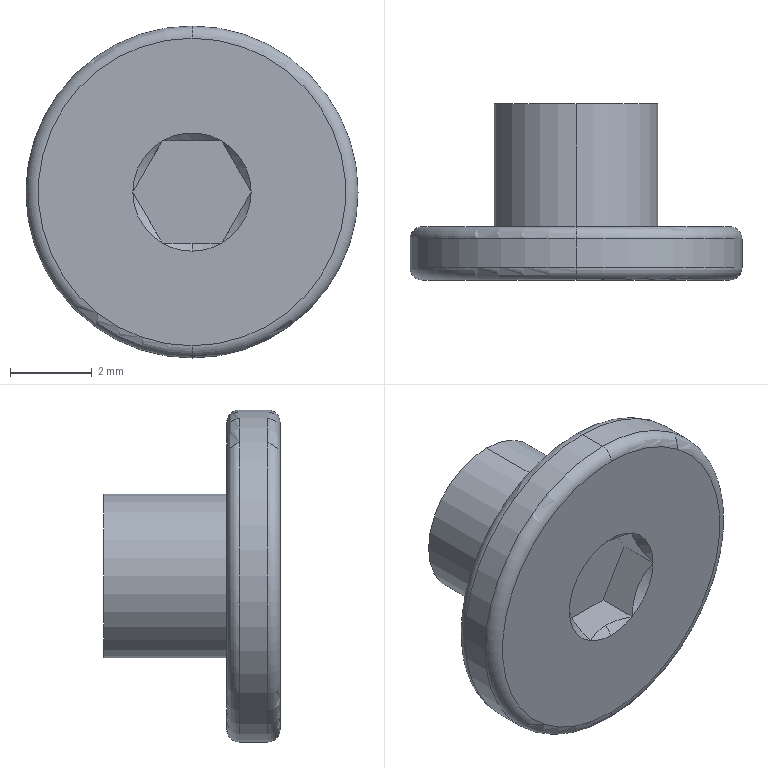Part | NX | features BREP 1 | 1 solid | 25 faces | box 8.1 x 4.3 x 8.1 mm | volume 98.194 mm3 | plane 10 | cone 7 | torus 4 | cylinder 4 | commonest cylinder face diameters 4 x2 8.1 x2
STEP:
#1=CARTESIAN_POINT('',(0.,0.1934,-1.25));
#2=VERTEX_POINT('',#1);
#3=CARTESIAN_POINT('',(0.7217,0.,-1.25));
#4=VERTEX_POINT('',#3);
#5=CARTESIAN_POINT('',(0.,0.1934,-1.25));
#6=CARTESIAN_POINT('',(0.2534,0.1934,-1.25));
#7=CARTESIAN_POINT('',(0.4959,0.1129,-1.25));
#8=CARTESIAN_POINT('',(0.7217,0.,-1.25));
#9=B_SPLINE_CURVE_WITH_KNOTS('',3,(#5,#6,#7,#8),.UNSPECIFIED.,.F.,.F.,(4,4),(0.,0.0007491),.UNSPECIFIED.);
#10=EDGE_CURVE('',#2,#4,#9,.T.);
#11=ORIENTED_EDGE('',*,*,#10,.F.);
#12=CARTESIAN_POINT('',(0.,0.,-1.443));
#13=VERTEX_POINT('',#12);
#14=CARTESIAN_POINT('',(0.,0.,-1.443));
#15=DIRECTION('',(0.,-0.7071,-0.7071));
#16=VECTOR('',#15,1000.);
#17=LINE('',#14,#16);
#18=EDGE_CURVE('',#2,#13,#17,.T.);
#19=ORIENTED_EDGE('',*,*,#18,.T.);
#20=CARTESIAN_POINT('',(0.,0.,0.));
#21=DIRECTION('',(0.,-1.,0.));
#22=DIRECTION('',(0.,0.,-1.));
#23=AXIS2_PLACEMENT_3D('',#20,#21,#22);
#24=CIRCLE('',#23,1.443);
#25=EDGE_CURVE('',#13,#4,#24,.T.);
#26=ORIENTED_EDGE('',*,*,#25,.T.);
#27=EDGE_LOOP('',(#11,#19,#26));
#28=FACE_BOUND('',#27,.T.);
#29=CARTESIAN_POINT('',(0.,0.,0.));
#30=DIRECTION('',(0.,-1.,0.));
#31=DIRECTION('',(0.,0.,1.));
#32=AXIS2_PLACEMENT_3D('',#29,#30,#31);
#33=CONICAL_SURFACE('',#32,1.443,0.7854);
#34=ADVANCED_FACE('',(#28),#33,.F.);
#35=CARTESIAN_POINT('',(0.,1.,-4.05));
#36=VERTEX_POINT('',#35);
#37=CARTESIAN_POINT('',(0.,1.,4.05));
#38=VERTEX_POINT('',#37);
#39=CARTESIAN_POINT('',(0.,1.,0.));
#40=DIRECTION('',(0.,-1.,0.));
#41=DIRECTION('',(0.,0.,1.));
#42=AXIS2_PLACEMENT_3D('',#39,#40,#41);
#43=CIRCLE('',#42,4.05);
#44=EDGE_CURVE('',#36,#38,#43,.T.);
#45=ORIENTED_EDGE('',*,*,#44,.F.);
#46=CARTESIAN_POINT('',(0.,1.3,-3.75));
#47=VERTEX_POINT('',#46);
#48=CARTESIAN_POINT('',(0.,1.,-3.75));
#49=DIRECTION('',(1.,0.,0.));
#50=DIRECTION('',(0.,0.,-1.));
#51=AXIS2_PLACEMENT_3D('',#48,#49,#50);
#52=CIRCLE('',#51,0.3);
#53=EDGE_CURVE('',#36,#47,#52,.T.);
#54=ORIENTED_EDGE('',*,*,#53,.T.);
#55=CARTESIAN_POINT('',(0.,1.3,3.75));
#56=VERTEX_POINT('',#55);
#57=CARTESIAN_POINT('',(0.,1.3,0.));
#58=DIRECTION('',(0.,1.,0.));
#59=DIRECTION('',(0.,0.,1.));
#60=AXIS2_PLACEMENT_3D('',#57,#58,#59);
#61=CIRCLE('',#60,3.75);
#62=EDGE_CURVE('',#56,#47,#61,.T.);
#63=ORIENTED_EDGE('',*,*,#62,.F.);
#64=CARTESIAN_POINT('',(0.,1.,3.75));
#65=DIRECTION('',(-1.,0.,0.));
#66=DIRECTION('',(0.,0.,1.));
#67=AXIS2_PLACEMENT_3D('',#64,#65,#66);
#68=CIRCLE('',#67,0.3);
#69=EDGE_CURVE('',#38,#56,#68,.T.);
#70=ORIENTED_EDGE('',*,*,#69,.F.);
#71=EDGE_LOOP('',(#45,#54,#63,#70));
#72=FACE_BOUND('',#71,.T.);
#73=CARTESIAN_POINT('',(0.,1.,0.));
#74=DIRECTION('',(0.,1.,0.));
#75=DIRECTION('',(0.,0.,-1.));
#76=AXIS2_PLACEMENT_3D('',#73,#74,#75);
#77=TOROIDAL_SURFACE('',#76,3.75,0.3);
#78=ADVANCED_FACE('',(#72),#77,.T.);
#79=CARTESIAN_POINT('',(0.,0.,-3.75));
#80=VERTEX_POINT('',#79);
#81=CARTESIAN_POINT('',(0.,0.,3.75));
#82=VERTEX_POINT('',#81);
#83=CARTESIAN_POINT('',(0.,0.,0.));
#84=DIRECTION('',(0.,-1.,0.));
#85=DIRECTION('',(0.,0.,1.));
#86=AXIS2_PLACEMENT_3D('',#83,#84,#85);
#87=CIRCLE('',#86,3.75);
#88=EDGE_CURVE('',#80,#82,#87,.T.);
#89=ORIENTED_EDGE('',*,*,#88,.F.);
#90=CARTESIAN_POINT('',(0.,0.3,-4.05));
#91=VERTEX_POINT('',#90);
#92=CARTESIAN_POINT('',(0.,0.3,-3.75));
#93=DIRECTION('',(1.,0.,0.));
#94=DIRECTION('',(0.,0.,-1.));
#95=AXIS2_PLACEMENT_3D('',#92,#93,#94);
#96=CIRCLE('',#95,0.3);
#97=EDGE_CURVE('',#80,#91,#96,.T.);
#98=ORIENTED_EDGE('',*,*,#97,.T.);
#99=CARTESIAN_POINT('',(0.,0.3,4.05));
#100=VERTEX_POINT('',#99);
#101=CARTESIAN_POINT('',(0.,0.3,0.));
#102=DIRECTION('',(0.,1.,0.));
#103=DIRECTION('',(0.,0.,1.));
#104=AXIS2_PLACEMENT_3D('',#101,#102,#103);
#105=CIRCLE('',#104,4.05);
#106=EDGE_CURVE('',#100,#91,#105,.T.);
#107=ORIENTED_EDGE('',*,*,#106,.F.);
#108=CARTESIAN_POINT('',(0.,0.3,3.75));
#109=DIRECTION('',(-1.,0.,0.));
#110=DIRECTION('',(0.,0.,1.));
#111=AXIS2_PLACEMENT_3D('',#108,#109,#110);
#112=CIRCLE('',#111,0.3);
#113=EDGE_CURVE('',#82,#100,#112,.T.);
#114=ORIENTED_EDGE('',*,*,#113,.F.);
#115=EDGE_LOOP('',(#89,#98,#107,#114));
#116=FACE_BOUND('',#115,.T.);
#117=CARTESIAN_POINT('',(0.,0.3,0.));
#118=DIRECTION('',(0.,1.,0.));
#119=DIRECTION('',(0.,0.,-1.));
#120=AXIS2_PLACEMENT_3D('',#117,#118,#119);
#121=TOROIDAL_SURFACE('',#120,3.75,0.3);
#122=ADVANCED_FACE('',(#116),#121,.T.);
#123=CARTESIAN_POINT('',(0.,4.3,2.));
#124=VERTEX_POINT('',#123);
#125=CARTESIAN_POINT('',(0.,4.3,-2.));
#126=VERTEX_POINT('',#125);
#127=CARTESIAN_POINT('',(0.,4.3,0.));
#128=DIRECTION('',(0.,1.,0.));
#129=DIRECTION('',(0.,0.,1.));
#130=AXIS2_PLACEMENT_3D('',#127,#128,#129);
#131=CIRCLE('',#130,2.);
#132=EDGE_CURVE('',#124,#126,#131,.T.);
#133=ORIENTED_EDGE('',*,*,#132,.F.);
#134=CARTESIAN_POINT('',(0.,1.3,2.));
#135=VERTEX_POINT('',#134);
#136=CARTESIAN_POINT('',(0.,4.3,2.));
#137=DIRECTION('',(0.,-1.,0.));
#138=VECTOR('',#137,1000.);
#139=LINE('',#136,#138);
#140=EDGE_CURVE('',#135,#124,#139,.F.);
#141=ORIENTED_EDGE('',*,*,#140,.F.);
#142=CARTESIAN_POINT('',(0.,1.3,-2.));
#143=VERTEX_POINT('',#142);
#144=CARTESIAN_POINT('',(0.,1.3,0.));
#145=DIRECTION('',(0.,1.,0.));
#146=DIRECTION('',(0.,0.,1.));
#147=AXIS2_PLACEMENT_3D('',#144,#145,#146);
#148=CIRCLE('',#147,2.);
#149=EDGE_CURVE('',#135,#143,#148,.T.);
#150=ORIENTED_EDGE('',*,*,#149,.T.);
#151=CARTESIAN_POINT('',(0.,4.3,-2.));
#152=DIRECTION('',(0.,-1.,0.));
#153=VECTOR('',#152,1000.);
#154=LINE('',#151,#153);
#155=EDGE_CURVE('',#143,#126,#154,.F.);
#156=ORIENTED_EDGE('',*,*,#155,.T.);
#157=EDGE_LOOP('',(#133,#141,#150,#156));
#158=FACE_BOUND('',#157,.T.);
#159=CARTESIAN_POINT('',(0.,4.3,0.));
#160=DIRECTION('',(0.,-1.,0.));
#161=DIRECTION('',(0.,0.,1.));
#162=AXIS2_PLACEMENT_3D('',#159,#160,#161);
#163=CYLINDRICAL_SURFACE('',#162,2.);
#164=ADVANCED_FACE('',(#158),#163,.T.);
#165=ORIENTED_EDGE('',*,*,#44,.T.);
#166=CARTESIAN_POINT('',(0.,1.3,4.05));
#167=DIRECTION('',(0.,-1.,0.));
#168=VECTOR('',#167,1000.);
#169=LINE('',#166,#168);
#170=EDGE_CURVE('',#100,#38,#169,.F.);
#171=ORIENTED_EDGE('',*,*,#170,.F.);
#172=ORIENTED_EDGE('',*,*,#106,.T.);
#173=CARTESIAN_POINT('',(0.,1.3,-4.05));
#174=DIRECTION('',(0.,-1.,0.));
#175=VECTOR('',#174,1000.);
#176=LINE('',#173,#175);
#177=EDGE_CURVE('',#91,#36,#176,.F.);
#178=ORIENTED_EDGE('',*,*,#177,.T.);
#179=EDGE_LOOP('',(#165,#171,#172,#178));
#180=FACE_BOUND('',#179,.T.);
#181=CARTESIAN_POINT('',(0.,1.3,0.));
#182=DIRECTION('',(0.,-1.,0.));
#183=DIRECTION('',(0.,0.,1.));
#184=AXIS2_PLACEMENT_3D('',#181,#182,#183);
#185=CYLINDRICAL_SURFACE('',#184,4.05);
#186=ADVANCED_FACE('',(#180),#185,.T.);
#187=ORIENTED_EDGE('',*,*,#170,.T.);
#188=CARTESIAN_POINT('',(0.,1.,0.));
#189=DIRECTION('',(0.,-1.,0.));
#190=DIRECTION('',(0.,0.,1.));
#191=AXIS2_PLACEMENT_3D('',#188,#189,#190);
#192=CIRCLE('',#191,4.05);
#193=EDGE_CURVE('',#38,#36,#192,.T.);
#194=ORIENTED_EDGE('',*,*,#193,.T.);
#195=ORIENTED_EDGE('',*,*,#177,.F.);
#196=CARTESIAN_POINT('',(0.,0.3,0.));
#197=DIRECTION('',(0.,1.,0.));
#198=DIRECTION('',(0.,0.,1.));
#199=AXIS2_PLACEMENT_3D('',#196,#197,#198);
#200=CIRCLE('',#199,4.05);
#201=EDGE_CURVE('',#91,#100,#200,.T.);
#202=ORIENTED_EDGE('',*,*,#201,.T.);
#203=EDGE_LOOP('',(#187,#194,#195,#202));
#204=FACE_BOUND('',#203,.T.);
#205=CARTESIAN_POINT('',(0.,1.3,0.));
#206=DIRECTION('',(0.,-1.,0.));
#207=DIRECTION('',(0.,0.,1.));
#208=AXIS2_PLACEMENT_3D('',#205,#206,#207);
#209=CYLINDRICAL_SURFACE('',#208,4.05);
#210=ADVANCED_FACE('',(#204),#209,.T.);
#211=ORIENTED_EDGE('',*,*,#62,.T.);
#212=CARTESIAN_POINT('',(0.,1.3,0.));
#213=DIRECTION('',(0.,1.,0.));
#214=DIRECTION('',(0.,0.,1.));
#215=AXIS2_PLACEMENT_3D('',#212,#213,#214);
#216=CIRCLE('',#215,3.75);
#217=EDGE_CURVE('',#47,#56,#216,.T.);
#218=ORIENTED_EDGE('',*,*,#217,.T.);
#219=EDGE_LOOP('',(#211,#218));
#220=FACE_BOUND('',#219,.T.);
#221=CARTESIAN_POINT('',(0.,1.3,0.));
#222=DIRECTION('',(0.,1.,0.));
#223=DIRECTION('',(0.,0.,1.));
#224=AXIS2_PLACEMENT_3D('',#221,#222,#223);
#225=CIRCLE('',#224,2.);
#226=EDGE_CURVE('',#143,#135,#225,.T.);
#227=ORIENTED_EDGE('',*,*,#226,.F.);
#228=ORIENTED_EDGE('',*,*,#149,.F.);
#229=EDGE_LOOP('',(#227,#228));
#230=FACE_BOUND('',#229,.T.);
#231=CARTESIAN_POINT('',(0.,1.3,0.));
#232=DIRECTION('',(0.,1.,0.));
#233=DIRECTION('',(-1.,0.,0.));
#234=AXIS2_PLACEMENT_3D('',#231,#232,#233);
#235=PLANE('',#234);
#236=ADVANCED_FACE('',(#220,#230),#235,.T.);
#237=CARTESIAN_POINT('',(0.,0.,0.));
#238=DIRECTION('',(0.,-1.,0.));
#239=DIRECTION('',(0.,0.,1.));
#240=AXIS2_PLACEMENT_3D('',#237,#238,#239);
#241=CIRCLE('',#240,3.75);
#242=EDGE_CURVE('',#82,#80,#241,.T.);
#243=ORIENTED_EDGE('',*,*,#242,.T.);
#244=ORIENTED_EDGE('',*,*,#88,.T.);
#245=EDGE_LOOP('',(#243,#244));
#246=FACE_BOUND('',#245,.T.);
#247=CARTESIAN_POINT('',(0.7217,0.,1.25));
#248=VERTEX_POINT('',#247);
#249=CARTESIAN_POINT('',(-0.7217,0.,1.25));
#250=VERTEX_POINT('',#249);
#251=CARTESIAN_POINT('',(0.,0.,0.));
#252=DIRECTION('',(0.,-1.,0.));
#253=DIRECTION('',(0.,0.,-1.));
#254=AXIS2_PLACEMENT_3D('',#251,#252,#253);
#255=CIRCLE('',#254,1.443);
#256=EDGE_CURVE('',#248,#250,#255,.T.);
#257=ORIENTED_EDGE('',*,*,#256,.F.);
#258=CARTESIAN_POINT('',(1.443,0.,0.));
#259=VERTEX_POINT('',#258);
#260=CARTESIAN_POINT('',(0.,0.,0.));
#261=DIRECTION('',(0.,-1.,0.));
#262=DIRECTION('',(0.,0.,-1.));
#263=AXIS2_PLACEMENT_3D('',#260,#261,#262);
#264=CIRCLE('',#263,1.443);
#265=EDGE_CURVE('',#259,#248,#264,.T.);
#266=ORIENTED_EDGE('',*,*,#265,.F.);
#267=CARTESIAN_POINT('',(0.,0.,0.));
#268=DIRECTION('',(0.,-1.,0.));
#269=DIRECTION('',(0.,0.,-1.));
#270=AXIS2_PLACEMENT_3D('',#267,#268,#269);
#271=CIRCLE('',#270,1.443);
#272=EDGE_CURVE('',#4,#259,#271,.T.);
#273=ORIENTED_EDGE('',*,*,#272,.F.);
#274=ORIENTED_EDGE('',*,*,#25,.F.);
#275=CARTESIAN_POINT('',(-0.7217,0.,-1.25));
#276=VERTEX_POINT('',#275);
#277=CARTESIAN_POINT('',(0.,0.,0.));
#278=DIRECTION('',(0.,-1.,0.));
#279=DIRECTION('',(0.,0.,-1.));
#280=AXIS2_PLACEMENT_3D('',#277,#278,#279);
#281=CIRCLE('',#280,1.443);
#282=EDGE_CURVE('',#276,#13,#281,.T.);
#283=ORIENTED_EDGE('',*,*,#282,.F.);
#284=CARTESIAN_POINT('',(-1.443,0.,0.));
#285=VERTEX_POINT('',#284);
#286=CARTESIAN_POINT('',(0.,0.,0.));
#287=DIRECTION('',(0.,-1.,0.));
#288=DIRECTION('',(0.,0.,-1.));
#289=AXIS2_PLACEMENT_3D('',#286,#287,#288);
#290=CIRCLE('',#289,1.443);
#291=EDGE_CURVE('',#285,#276,#290,.T.);
#292=ORIENTED_EDGE('',*,*,#291,.F.);
#293=CARTESIAN_POINT('',(0.,0.,0.));
#294=DIRECTION('',(0.,-1.,0.));
#295=DIRECTION('',(0.,0.,-1.));
#296=AXIS2_PLACEMENT_3D('',#293,#294,#295);
#297=CIRCLE('',#296,1.443);
#298=EDGE_CURVE('',#250,#285,#297,.T.);
#299=ORIENTED_EDGE('',*,*,#298,.F.);
#300=EDGE_LOOP('',(#257,#266,#273,#274,#283,#292,#299));
#301=FACE_BOUND('',#300,.T.);
#302=CARTESIAN_POINT('',(0.,0.,0.));
#303=DIRECTION('',(0.,1.,0.));
#304=DIRECTION('',(-1.,0.,0.));
#305=AXIS2_PLACEMENT_3D('',#302,#303,#304);
#306=PLANE('',#305);
#307=ADVANCED_FACE('',(#246,#301),#306,.F.);
#308=ORIENTED_EDGE('',*,*,#140,.T.);
#309=CARTESIAN_POINT('',(0.,4.3,0.));
#310=DIRECTION('',(0.,1.,0.));
#311=DIRECTION('',(0.,0.,1.));
#312=AXIS2_PLACEMENT_3D('',#309,#310,#311);
#313=CIRCLE('',#312,2.);
#314=EDGE_CURVE('',#126,#124,#313,.T.);
#315=ORIENTED_EDGE('',*,*,#314,.F.);
#316=ORIENTED_EDGE('',*,*,#155,.F.);
#317=ORIENTED_EDGE('',*,*,#226,.T.);
#318=EDGE_LOOP('',(#308,#315,#316,#317));
#319=FACE_BOUND('',#318,.T.);
#320=CARTESIAN_POINT('',(0.,4.3,0.));
#321=DIRECTION('',(0.,-1.,0.));
#322=DIRECTION('',(0.,0.,1.));
#323=AXIS2_PLACEMENT_3D('',#320,#321,#322);
#324=CYLINDRICAL_SURFACE('',#323,2.);
#325=ADVANCED_FACE('',(#319),#324,.T.);
#326=ORIENTED_EDGE('',*,*,#314,.T.);
#327=ORIENTED_EDGE('',*,*,#132,.T.);
#328=EDGE_LOOP('',(#326,#327));
#329=FACE_BOUND('',#328,.T.);
#330=CARTESIAN_POINT('',(0.,4.3,0.));
#331=DIRECTION('',(0.,1.,0.));
#332=DIRECTION('',(-1.,0.,0.));
#333=AXIS2_PLACEMENT_3D('',#330,#331,#332);
#334=PLANE('',#333);
#335=ADVANCED_FACE('',(#329),#334,.T.);
#336=ORIENTED_EDGE('',*,*,#97,.F.);
#337=ORIENTED_EDGE('',*,*,#242,.F.);
#338=ORIENTED_EDGE('',*,*,#113,.T.);
#339=ORIENTED_EDGE('',*,*,#201,.F.);
#340=EDGE_LOOP('',(#336,#337,#338,#339));
#341=FACE_BOUND('',#340,.T.);
#342=CARTESIAN_POINT('',(0.,0.3,0.));
#343=DIRECTION('',(0.,1.,0.));
#344=DIRECTION('',(0.,0.,-1.));
#345=AXIS2_PLACEMENT_3D('',#342,#343,#344);
#346=TOROIDAL_SURFACE('',#345,3.75,0.3);
#347=ADVANCED_FACE('',(#341),#346,.T.);
#348=ORIENTED_EDGE('',*,*,#53,.F.);
#349=ORIENTED_EDGE('',*,*,#193,.F.);
#350=ORIENTED_EDGE('',*,*,#69,.T.);
#351=ORIENTED_EDGE('',*,*,#217,.F.);
#352=EDGE_LOOP('',(#348,#349,#350,#351));
#353=FACE_BOUND('',#352,.T.);
#354=CARTESIAN_POINT('',(0.,1.,0.));
#355=DIRECTION('',(0.,1.,0.));
#356=DIRECTION('',(0.,0.,-1.));
#357=AXIS2_PLACEMENT_3D('',#354,#355,#356);
#358=TOROIDAL_SURFACE('',#357,3.75,0.3);
#359=ADVANCED_FACE('',(#353),#358,.T.);
#360=ORIENTED_EDGE('',*,*,#265,.T.);
#361=CARTESIAN_POINT('',(1.443,0.,0.));
#362=CARTESIAN_POINT('',(1.218,0.2255,0.3907));
#363=CARTESIAN_POINT('',(0.9486,0.2269,0.857));
#364=CARTESIAN_POINT('',(0.7217,0.,1.25));
#365=B_SPLINE_CURVE_WITH_KNOTS('',3,(#361,#362,#363,#364),.UNSPECIFIED.,.F.,.F.,(4,4),(0.,0.001491),.UNSPECIFIED.);
#366=EDGE_CURVE('',#259,#248,#365,.T.);
#367=ORIENTED_EDGE('',*,*,#366,.F.);
#368=EDGE_LOOP('',(#360,#367));
#369=FACE_BOUND('',#368,.T.);
#370=CARTESIAN_POINT('',(0.,0.,0.));
#371=DIRECTION('',(0.,-1.,0.));
#372=DIRECTION('',(0.,0.,1.));
#373=AXIS2_PLACEMENT_3D('',#370,#371,#372);
#374=CONICAL_SURFACE('',#373,1.443,0.7854);
#375=ADVANCED_FACE('',(#369),#374,.F.);
#376=ORIENTED_EDGE('',*,*,#256,.T.);
#377=CARTESIAN_POINT('',(0.7217,0.,1.25));
#378=CARTESIAN_POINT('',(0.2706,0.2255,1.25));
#379=CARTESIAN_POINT('',(-0.2679,0.2269,1.25));
#380=CARTESIAN_POINT('',(-0.7217,0.,1.25));
#381=B_SPLINE_CURVE_WITH_KNOTS('',3,(#377,#378,#379,#380),.UNSPECIFIED.,.F.,.F.,(4,4),(0.,0.001491),.UNSPECIFIED.);
#382=EDGE_CURVE('',#248,#250,#381,.T.);
#383=ORIENTED_EDGE('',*,*,#382,.F.);
#384=EDGE_LOOP('',(#376,#383));
#385=FACE_BOUND('',#384,.T.);
#386=CARTESIAN_POINT('',(0.,0.,0.));
#387=DIRECTION('',(0.,-1.,0.));
#388=DIRECTION('',(0.,0.,1.));
#389=AXIS2_PLACEMENT_3D('',#386,#387,#388);
#390=CONICAL_SURFACE('',#389,1.443,0.7854);
#391=ADVANCED_FACE('',(#385),#390,.F.);
#392=ORIENTED_EDGE('',*,*,#298,.T.);
#393=CARTESIAN_POINT('',(-0.7217,0.,1.25));
#394=CARTESIAN_POINT('',(-0.9472,0.2255,0.8593));
#395=CARTESIAN_POINT('',(-1.216,0.2269,0.393));
#396=CARTESIAN_POINT('',(-1.443,0.,0.));
#397=B_SPLINE_CURVE_WITH_KNOTS('',3,(#393,#394,#395,#396),.UNSPECIFIED.,.F.,.F.,(4,4),(0.,0.001491),.UNSPECIFIED.);
#398=EDGE_CURVE('',#250,#285,#397,.T.);
#399=ORIENTED_EDGE('',*,*,#398,.F.);
#400=EDGE_LOOP('',(#392,#399));
#401=FACE_BOUND('',#400,.T.);
#402=CARTESIAN_POINT('',(0.,0.,0.));
#403=DIRECTION('',(0.,-1.,0.));
#404=DIRECTION('',(0.,0.,1.));
#405=AXIS2_PLACEMENT_3D('',#402,#403,#404);
#406=CONICAL_SURFACE('',#405,1.443,0.7854);
#407=ADVANCED_FACE('',(#401),#406,.F.);
#408=ORIENTED_EDGE('',*,*,#291,.T.);
#409=CARTESIAN_POINT('',(-1.443,0.,0.));
#410=CARTESIAN_POINT('',(-1.218,0.2255,-0.3907));
#411=CARTESIAN_POINT('',(-0.9486,0.2269,-0.857));
#412=CARTESIAN_POINT('',(-0.7217,0.,-1.25));
#413=B_SPLINE_CURVE_WITH_KNOTS('',3,(#409,#410,#411,#412),.UNSPECIFIED.,.F.,.F.,(4,4),(0.,0.001491),.UNSPECIFIED.);
#414=EDGE_CURVE('',#285,#276,#413,.T.);
#415=ORIENTED_EDGE('',*,*,#414,.F.);
#416=EDGE_LOOP('',(#408,#415));
#417=FACE_BOUND('',#416,.T.);
#418=CARTESIAN_POINT('',(0.,0.,0.));
#419=DIRECTION('',(0.,-1.,0.));
#420=DIRECTION('',(0.,0.,1.));
#421=AXIS2_PLACEMENT_3D('',#418,#419,#420);
#422=CONICAL_SURFACE('',#421,1.443,0.7854);
#423=ADVANCED_FACE('',(#417),#422,.F.);
#424=ORIENTED_EDGE('',*,*,#18,.F.);
#425=CARTESIAN_POINT('',(-0.7217,0.,-1.25));
#426=CARTESIAN_POINT('',(-0.4955,0.1131,-1.25));
#427=CARTESIAN_POINT('',(-0.2554,0.1934,-1.25));
#428=CARTESIAN_POINT('',(0.,0.1934,-1.25));
#429=B_SPLINE_CURVE_WITH_KNOTS('',3,(#425,#426,#427,#428),.UNSPECIFIED.,.F.,.F.,(4,4),(0.,0.0007476),.UNSPECIFIED.);
#430=EDGE_CURVE('',#276,#2,#429,.T.);
#431=ORIENTED_EDGE('',*,*,#430,.F.);
#432=ORIENTED_EDGE('',*,*,#282,.T.);
#433=EDGE_LOOP('',(#424,#431,#432));
#434=FACE_BOUND('',#433,.T.);
#435=CARTESIAN_POINT('',(0.,0.,0.));
#436=DIRECTION('',(0.,-1.,0.));
#437=DIRECTION('',(0.,0.,1.));
#438=AXIS2_PLACEMENT_3D('',#435,#436,#437);
#439=CONICAL_SURFACE('',#438,1.443,0.7854);
#440=ADVANCED_FACE('',(#434),#439,.F.);
#441=ORIENTED_EDGE('',*,*,#272,.T.);
#442=CARTESIAN_POINT('',(0.7217,0.,-1.25));
#443=CARTESIAN_POINT('',(0.9472,0.2255,-0.8593));
#444=CARTESIAN_POINT('',(1.216,0.2269,-0.393));
#445=CARTESIAN_POINT('',(1.443,0.,0.));
#446=B_SPLINE_CURVE_WITH_KNOTS('',3,(#442,#443,#444,#445),.UNSPECIFIED.,.F.,.F.,(4,4),(0.,0.001491),.UNSPECIFIED.);
#447=EDGE_CURVE('',#4,#259,#446,.T.);
#448=ORIENTED_EDGE('',*,*,#447,.F.);
#449=EDGE_LOOP('',(#441,#448));
#450=FACE_BOUND('',#449,.T.);
#451=CARTESIAN_POINT('',(0.,0.,0.));
#452=DIRECTION('',(0.,-1.,0.));
#453=DIRECTION('',(0.,0.,1.));
#454=AXIS2_PLACEMENT_3D('',#451,#452,#453);
#455=CONICAL_SURFACE('',#454,1.443,0.7854);
#456=ADVANCED_FACE('',(#450),#455,.F.);
#457=CARTESIAN_POINT('',(0.7217,1.,-1.25));
#458=VERTEX_POINT('',#457);
#459=CARTESIAN_POINT('',(1.443,1.,0.));
#460=VERTEX_POINT('',#459);
#461=CARTESIAN_POINT('',(0.7217,1.,-1.25));
#462=DIRECTION('',(0.5,0.,0.866));
#463=VECTOR('',#462,1000.);
#464=LINE('',#461,#463);
#465=EDGE_CURVE('',#458,#460,#464,.T.);
#466=ORIENTED_EDGE('',*,*,#465,.T.);
#467=CARTESIAN_POINT('',(0.7217,1.,1.25));
#468=VERTEX_POINT('',#467);
#469=CARTESIAN_POINT('',(1.443,1.,0.));
#470=DIRECTION('',(-0.5,0.,0.866));
#471=VECTOR('',#470,1000.);
#472=LINE('',#469,#471);
#473=EDGE_CURVE('',#460,#468,#472,.T.);
#474=ORIENTED_EDGE('',*,*,#473,.T.);
#475=CARTESIAN_POINT('',(-0.7217,1.,1.25));
#476=VERTEX_POINT('',#475);
#477=CARTESIAN_POINT('',(0.7217,1.,1.25));
#478=DIRECTION('',(-1.,0.,0.));
#479=VECTOR('',#478,1000.);
#480=LINE('',#477,#479);
#481=EDGE_CURVE('',#468,#476,#480,.T.);
#482=ORIENTED_EDGE('',*,*,#481,.T.);
#483=CARTESIAN_POINT('',(-1.443,1.,0.));
#484=VERTEX_POINT('',#483);
#485=CARTESIAN_POINT('',(-0.7217,1.,1.25));
#486=DIRECTION('',(-0.5,0.,-0.866));
#487=VECTOR('',#486,1000.);
#488=LINE('',#485,#487);
#489=EDGE_CURVE('',#476,#484,#488,.T.);
#490=ORIENTED_EDGE('',*,*,#489,.T.);
#491=CARTESIAN_POINT('',(-0.7217,1.,-1.25));
#492=VERTEX_POINT('',#491);
#493=CARTESIAN_POINT('',(-1.443,1.,0.));
#494=DIRECTION('',(0.5,0.,-0.866));
#495=VECTOR('',#494,1000.);
#496=LINE('',#493,#495);
#497=EDGE_CURVE('',#484,#492,#496,.T.);
#498=ORIENTED_EDGE('',*,*,#497,.T.);
#499=CARTESIAN_POINT('',(-0.7217,1.,-1.25));
#500=DIRECTION('',(1.,0.,0.));
#501=VECTOR('',#500,1000.);
#502=LINE('',#499,#501);
#503=EDGE_CURVE('',#492,#458,#502,.T.);
#504=ORIENTED_EDGE('',*,*,#503,.T.);
#505=EDGE_LOOP('',(#466,#474,#482,#490,#498,#504));
#506=FACE_BOUND('',#505,.T.);
#507=CARTESIAN_POINT('',(0.,1.,0.));
#508=DIRECTION('',(0.,-1.,0.));
#509=DIRECTION('',(0.,0.,1.));
#510=AXIS2_PLACEMENT_3D('',#507,#508,#509);
#511=PLANE('',#510);
#512=ADVANCED_FACE('',(#506),#511,.T.);
#513=CARTESIAN_POINT('',(1.443,1.,0.));
#514=DIRECTION('',(0.,-1.,0.));
#515=VECTOR('',#514,1000.);
#516=LINE('',#513,#515);
#517=EDGE_CURVE('',#460,#259,#516,.T.);
#518=ORIENTED_EDGE('',*,*,#517,.T.);
#519=ORIENTED_EDGE('',*,*,#366,.T.);
#520=CARTESIAN_POINT('',(0.7217,1.,1.25));
#521=DIRECTION('',(0.,-1.,0.));
#522=VECTOR('',#521,1000.);
#523=LINE('',#520,#522);
#524=EDGE_CURVE('',#468,#248,#523,.T.);
#525=ORIENTED_EDGE('',*,*,#524,.F.);
#526=ORIENTED_EDGE('',*,*,#473,.F.);
#527=EDGE_LOOP('',(#518,#519,#525,#526));
#528=FACE_BOUND('',#527,.T.);
#529=CARTESIAN_POINT('',(1.443,1.,0.));
#530=DIRECTION('',(0.866,0.,0.5));
#531=DIRECTION('',(0.,1.,0.));
#532=AXIS2_PLACEMENT_3D('',#529,#530,#531);
#533=PLANE('',#532);
#534=ADVANCED_FACE('',(#528),#533,.F.);
#535=ORIENTED_EDGE('',*,*,#524,.T.);
#536=ORIENTED_EDGE('',*,*,#382,.T.);
#537=CARTESIAN_POINT('',(-0.7217,1.,1.25));
#538=DIRECTION('',(0.,-1.,0.));
#539=VECTOR('',#538,1000.);
#540=LINE('',#537,#539);
#541=EDGE_CURVE('',#476,#250,#540,.T.);
#542=ORIENTED_EDGE('',*,*,#541,.F.);
#543=ORIENTED_EDGE('',*,*,#481,.F.);
#544=EDGE_LOOP('',(#535,#536,#542,#543));
#545=FACE_BOUND('',#544,.T.);
#546=CARTESIAN_POINT('',(0.7217,1.,1.25));
#547=DIRECTION('',(0.,0.,1.));
#548=DIRECTION('',(-1.,0.,0.));
#549=AXIS2_PLACEMENT_3D('',#546,#547,#548);
#550=PLANE('',#549);
#551=ADVANCED_FACE('',(#545),#550,.F.);
#552=ORIENTED_EDGE('',*,*,#541,.T.);
#553=ORIENTED_EDGE('',*,*,#398,.T.);
#554=CARTESIAN_POINT('',(-1.443,1.,0.));
#555=DIRECTION('',(0.,-1.,0.));
#556=VECTOR('',#555,1000.);
#557=LINE('',#554,#556);
#558=EDGE_CURVE('',#484,#285,#557,.T.);
#559=ORIENTED_EDGE('',*,*,#558,.F.);
#560=ORIENTED_EDGE('',*,*,#489,.F.);
#561=EDGE_LOOP('',(#552,#553,#559,#560));
#562=FACE_BOUND('',#561,.T.);
#563=CARTESIAN_POINT('',(-0.7217,1.,1.25));
#564=DIRECTION('',(-0.866,0.,0.5));
#565=DIRECTION('',(0.,-1.,0.));
#566=AXIS2_PLACEMENT_3D('',#563,#564,#565);
#567=PLANE('',#566);
#568=ADVANCED_FACE('',(#562),#567,.F.);
#569=ORIENTED_EDGE('',*,*,#558,.T.);
#570=ORIENTED_EDGE('',*,*,#414,.T.);
#571=CARTESIAN_POINT('',(-0.7217,1.,-1.25));
#572=DIRECTION('',(0.,-1.,0.));
#573=VECTOR('',#572,1000.);
#574=LINE('',#571,#573);
#575=EDGE_CURVE('',#492,#276,#574,.T.);
#576=ORIENTED_EDGE('',*,*,#575,.F.);
#577=ORIENTED_EDGE('',*,*,#497,.F.);
#578=EDGE_LOOP('',(#569,#570,#576,#577));
#579=FACE_BOUND('',#578,.T.);
#580=CARTESIAN_POINT('',(-1.443,1.,0.));
#581=DIRECTION('',(-0.866,0.,-0.5));
#582=DIRECTION('',(0.5,0.,-0.866));
#583=AXIS2_PLACEMENT_3D('',#580,#581,#582);
#584=PLANE('',#583);
#585=ADVANCED_FACE('',(#579),#584,.F.);
#586=ORIENTED_EDGE('',*,*,#575,.T.);
#587=ORIENTED_EDGE('',*,*,#430,.T.);
#588=ORIENTED_EDGE('',*,*,#10,.T.);
#589=CARTESIAN_POINT('',(0.7217,1.,-1.25));
#590=DIRECTION('',(0.,-1.,0.));
#591=VECTOR('',#590,1000.);
#592=LINE('',#589,#591);
#593=EDGE_CURVE('',#458,#4,#592,.T.);
#594=ORIENTED_EDGE('',*,*,#593,.F.);
#595=ORIENTED_EDGE('',*,*,#503,.F.);
#596=EDGE_LOOP('',(#586,#587,#588,#594,#595));
#597=FACE_BOUND('',#596,.T.);
#598=CARTESIAN_POINT('',(-0.7217,1.,-1.25));
#599=DIRECTION('',(0.,0.,-1.));
#600=DIRECTION('',(1.,0.,0.));
#601=AXIS2_PLACEMENT_3D('',#598,#599,#600);
#602=PLANE('',#601);
#603=ADVANCED_FACE('',(#597),#602,.F.);
#604=ORIENTED_EDGE('',*,*,#593,.T.);
#605=ORIENTED_EDGE('',*,*,#447,.T.);
#606=ORIENTED_EDGE('',*,*,#517,.F.);
#607=ORIENTED_EDGE('',*,*,#465,.F.);
#608=EDGE_LOOP('',(#604,#605,#606,#607));
#609=FACE_BOUND('',#608,.T.);
#610=CARTESIAN_POINT('',(0.7217,1.,-1.25));
#611=DIRECTION('',(0.866,0.,-0.5));
#612=DIRECTION('',(0.,1.,0.));
#613=AXIS2_PLACEMENT_3D('',#610,#611,#612);
#614=PLANE('',#613);
#615=ADVANCED_FACE('',(#609),#614,.F.);
#616=CLOSED_SHELL('',(#34,#78,#122,#164,#186,#210,#236,#307,#325,#335,#347,#359,#375,#391,#407,#423,#440,#456,#512,#534,#551,#568,#585,#603,#615));
#617=MANIFOLD_SOLID_BREP('',#616);
#618=(LENGTH_UNIT()NAMED_UNIT(*)SI_UNIT(.MILLI.,.METRE.));
#619=UNCERTAINTY_MEASURE_WITH_UNIT(LENGTH_MEASURE(0.0508),#618,'','');
#620=(NAMED_UNIT(*)PLANE_ANGLE_UNIT()SI_UNIT($,.RADIAN.));
#621=(NAMED_UNIT(*)SI_UNIT($,.STERADIAN.)SOLID_ANGLE_UNIT());
#622=(GEOMETRIC_REPRESENTATION_CONTEXT(3)GLOBAL_UNCERTAINTY_ASSIGNED_CONTEXT((#619))GLOBAL_UNIT_ASSIGNED_CONTEXT((#618,#620,#621))REPRESENTATION_CONTEXT('',''));
#623=ADVANCED_BREP_SHAPE_REPRESENTATION('',(#617),#622);